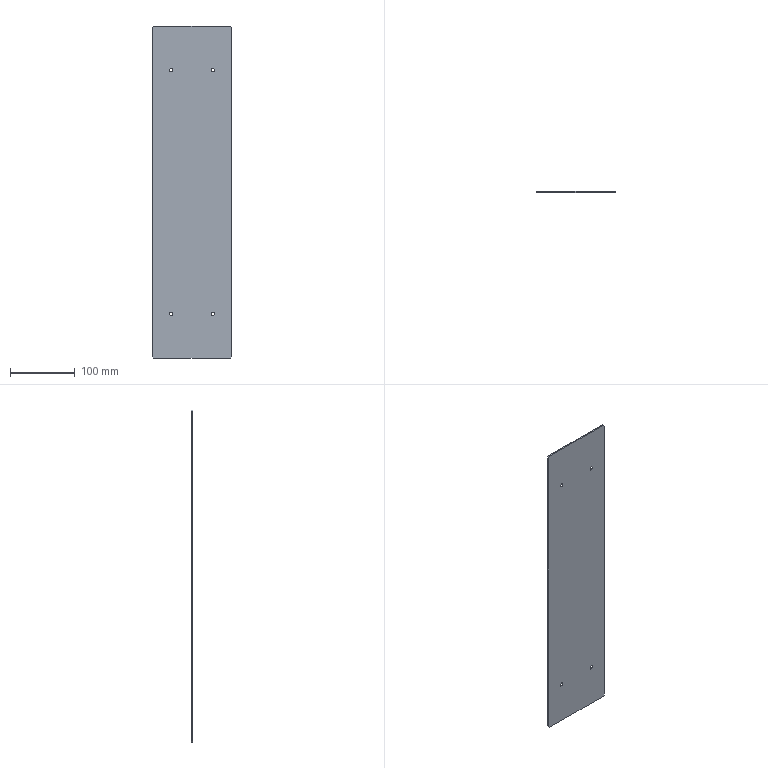Part | STEP file | (PA01.001.LX019) Cover Plate | 1 solid | 18 faces | box 123 x 2 x 511 mm | volume 125357 mm3 | plane 10 | cone 8
STEP:
#1=CARTESIAN_POINT('',(0.,0.,0.));
#2=DIRECTION('',(0.,0.,1.));
#3=DIRECTION('',(1.,0.,0.));
#4=AXIS2_PLACEMENT_3D('',#1,#2,#3);
#5=CARTESIAN_POINT('',(29.5,-2.,70.48));
#6=VERTEX_POINT('',#5);
#7=CARTESIAN_POINT('',(29.5,0.,72.48));
#8=VERTEX_POINT('',#7);
#9=CARTESIAN_POINT('',(29.5,0.,72.48));
#10=DIRECTION('',(0.,0.7071,0.7071));
#11=VECTOR('',#10,1.);
#12=LINE('',#9,#11);
#13=CARTESIAN_POINT('',(29.5,0.,68.));
#14=DIRECTION('',(0.,1.,0.));
#15=DIRECTION('',(0.,0.,1.));
#16=AXIS2_PLACEMENT_3D('',#13,#14,#15);
#17=CONICAL_SURFACE('',#16,4.48,0.7854);
#18=CARTESIAN_POINT('',(6.283,0.));
#19=DIRECTION('',(0.,1.));
#20=VECTOR('',#19,1.);
#21=LINE('',#18,#20);
#22=(GEOMETRIC_REPRESENTATION_CONTEXT(2)PARAMETRIC_REPRESENTATION_CONTEXT()REPRESENTATION_CONTEXT('',''));
#23=DEFINITIONAL_REPRESENTATION('',(#21),#22);
#24=PCURVE('',#17,#23);
#25=CARTESIAN_POINT('',(29.5,0.,68.));
#26=DIRECTION('',(0.,1.,0.));
#27=DIRECTION('',(0.,0.,1.));
#28=AXIS2_PLACEMENT_3D('',#25,#26,#27);
#29=CONICAL_SURFACE('',#28,4.48,0.7854);
#30=CARTESIAN_POINT('',(0.,0.));
#31=DIRECTION('',(0.,1.));
#32=VECTOR('',#31,1.);
#33=LINE('',#30,#32);
#34=(GEOMETRIC_REPRESENTATION_CONTEXT(2)PARAMETRIC_REPRESENTATION_CONTEXT()REPRESENTATION_CONTEXT('',''));
#35=DEFINITIONAL_REPRESENTATION('',(#33),#34);
#36=PCURVE('',#29,#35);
#37=SURFACE_CURVE('',#12,(#24,#36),.PCURVE_S1.);
#38=EDGE_CURVE('',#6,#8,#37,.T.);
#39=ORIENTED_EDGE('',*,*,#38,.T.);
#40=CARTESIAN_POINT('',(29.5,0.,63.52));
#41=VERTEX_POINT('',#40);
#42=CARTESIAN_POINT('',(29.5,0.,68.));
#43=DIRECTION('',(0.,1.,0.));
#44=DIRECTION('',(0.,0.,1.));
#45=AXIS2_PLACEMENT_3D('',#42,#43,#44);
#46=CIRCLE('',#45,4.48);
#47=CARTESIAN_POINT('',(0.,0.));
#48=DIRECTION('',(1.,0.));
#49=VECTOR('',#48,1.);
#50=LINE('',#47,#49);
#51=(GEOMETRIC_REPRESENTATION_CONTEXT(2)PARAMETRIC_REPRESENTATION_CONTEXT()REPRESENTATION_CONTEXT('',''));
#52=DEFINITIONAL_REPRESENTATION('',(#50),#51);
#53=PCURVE('',#17,#52);
#54=CARTESIAN_POINT('',(0.,0.,511.));
#55=DIRECTION('',(0.,1.,0.));
#56=DIRECTION('',(0.,0.,1.));
#57=AXIS2_PLACEMENT_3D('',#54,#55,#56);
#58=PLANE('',#57);
#59=CARTESIAN_POINT('',(-443.,29.5));
#60=DIRECTION('',(1.,0.));
#61=AXIS2_PLACEMENT_2D('',#59,#60);
#62=CIRCLE('',#61,4.48);
#63=(GEOMETRIC_REPRESENTATION_CONTEXT(2)PARAMETRIC_REPRESENTATION_CONTEXT()REPRESENTATION_CONTEXT('',''));
#64=DEFINITIONAL_REPRESENTATION('',(#62),#63);
#65=PCURVE('',#58,#64);
#66=SURFACE_CURVE('',#46,(#53,#65),.PCURVE_S1.);
#67=EDGE_CURVE('',#41,#8,#66,.T.);
#68=ORIENTED_EDGE('',*,*,#67,.F.);
#69=CARTESIAN_POINT('',(29.5,-2.,65.52));
#70=VERTEX_POINT('',#69);
#71=CARTESIAN_POINT('',(29.5,0.,63.52));
#72=DIRECTION('',(0.,0.7071,-0.7071));
#73=VECTOR('',#72,1.);
#74=LINE('',#71,#73);
#75=CARTESIAN_POINT('',(3.142,0.));
#76=DIRECTION('',(0.,1.));
#77=VECTOR('',#76,1.);
#78=LINE('',#75,#77);
#79=(GEOMETRIC_REPRESENTATION_CONTEXT(2)PARAMETRIC_REPRESENTATION_CONTEXT()REPRESENTATION_CONTEXT('',''));
#80=DEFINITIONAL_REPRESENTATION('',(#78),#79);
#81=PCURVE('',#17,#80);
#82=CARTESIAN_POINT('',(3.142,0.));
#83=DIRECTION('',(0.,1.));
#84=VECTOR('',#83,1.);
#85=LINE('',#82,#84);
#86=(GEOMETRIC_REPRESENTATION_CONTEXT(2)PARAMETRIC_REPRESENTATION_CONTEXT()REPRESENTATION_CONTEXT('',''));
#87=DEFINITIONAL_REPRESENTATION('',(#85),#86);
#88=PCURVE('',#29,#87);
#89=SURFACE_CURVE('',#74,(#81,#88),.PCURVE_S1.);
#90=EDGE_CURVE('',#70,#41,#89,.T.);
#91=ORIENTED_EDGE('',*,*,#90,.F.);
#92=CARTESIAN_POINT('',(29.5,-2.,68.));
#93=DIRECTION('',(0.,1.,0.));
#94=DIRECTION('',(0.,0.,1.));
#95=AXIS2_PLACEMENT_3D('',#92,#93,#94);
#96=CIRCLE('',#95,2.48);
#97=CARTESIAN_POINT('',(0.,-2.));
#98=DIRECTION('',(1.,0.));
#99=VECTOR('',#98,1.);
#100=LINE('',#97,#99);
#101=(GEOMETRIC_REPRESENTATION_CONTEXT(2)PARAMETRIC_REPRESENTATION_CONTEXT()REPRESENTATION_CONTEXT('',''));
#102=DEFINITIONAL_REPRESENTATION('',(#100),#101);
#103=PCURVE('',#17,#102);
#104=CARTESIAN_POINT('',(0.,-2.,511.));
#105=DIRECTION('',(0.,1.,0.));
#106=DIRECTION('',(0.,0.,1.));
#107=AXIS2_PLACEMENT_3D('',#104,#105,#106);
#108=PLANE('',#107);
#109=CARTESIAN_POINT('',(-443.,29.5));
#110=DIRECTION('',(1.,0.));
#111=AXIS2_PLACEMENT_2D('',#109,#110);
#112=CIRCLE('',#111,2.48);
#113=(GEOMETRIC_REPRESENTATION_CONTEXT(2)PARAMETRIC_REPRESENTATION_CONTEXT()REPRESENTATION_CONTEXT('',''));
#114=DEFINITIONAL_REPRESENTATION('',(#112),#113);
#115=PCURVE('',#108,#114);
#116=SURFACE_CURVE('',#96,(#103,#115),.PCURVE_S1.);
#117=EDGE_CURVE('',#70,#6,#116,.T.);
#118=ORIENTED_EDGE('',*,*,#117,.T.);
#119=EDGE_LOOP('',(#39,#68,#91,#118));
#120=FACE_BOUND('',#119,.F.);
#121=ADVANCED_FACE('',(#120),#17,.F.);
#122=CARTESIAN_POINT('',(93.5,-2.,70.48));
#123=VERTEX_POINT('',#122);
#124=CARTESIAN_POINT('',(93.5,0.,72.48));
#125=VERTEX_POINT('',#124);
#126=CARTESIAN_POINT('',(93.5,0.,72.48));
#127=DIRECTION('',(0.,0.7071,0.7071));
#128=VECTOR('',#127,1.);
#129=LINE('',#126,#128);
#130=CARTESIAN_POINT('',(93.5,0.,68.));
#131=DIRECTION('',(0.,1.,0.));
#132=DIRECTION('',(0.,0.,1.));
#133=AXIS2_PLACEMENT_3D('',#130,#131,#132);
#134=CONICAL_SURFACE('',#133,4.48,0.7854);
#135=CARTESIAN_POINT('',(6.283,0.));
#136=DIRECTION('',(0.,1.));
#137=VECTOR('',#136,1.);
#138=LINE('',#135,#137);
#139=(GEOMETRIC_REPRESENTATION_CONTEXT(2)PARAMETRIC_REPRESENTATION_CONTEXT()REPRESENTATION_CONTEXT('',''));
#140=DEFINITIONAL_REPRESENTATION('',(#138),#139);
#141=PCURVE('',#134,#140);
#142=CARTESIAN_POINT('',(93.5,0.,68.));
#143=DIRECTION('',(0.,1.,0.));
#144=DIRECTION('',(0.,0.,1.));
#145=AXIS2_PLACEMENT_3D('',#142,#143,#144);
#146=CONICAL_SURFACE('',#145,4.48,0.7854);
#147=CARTESIAN_POINT('',(0.,0.));
#148=DIRECTION('',(0.,1.));
#149=VECTOR('',#148,1.);
#150=LINE('',#147,#149);
#151=(GEOMETRIC_REPRESENTATION_CONTEXT(2)PARAMETRIC_REPRESENTATION_CONTEXT()REPRESENTATION_CONTEXT('',''));
#152=DEFINITIONAL_REPRESENTATION('',(#150),#151);
#153=PCURVE('',#146,#152);
#154=SURFACE_CURVE('',#129,(#141,#153),.PCURVE_S1.);
#155=EDGE_CURVE('',#123,#125,#154,.T.);
#156=ORIENTED_EDGE('',*,*,#155,.T.);
#157=CARTESIAN_POINT('',(93.5,0.,63.52));
#158=VERTEX_POINT('',#157);
#159=CARTESIAN_POINT('',(93.5,0.,68.));
#160=DIRECTION('',(0.,1.,0.));
#161=DIRECTION('',(0.,0.,1.));
#162=AXIS2_PLACEMENT_3D('',#159,#160,#161);
#163=CIRCLE('',#162,4.48);
#164=CARTESIAN_POINT('',(0.,0.));
#165=DIRECTION('',(1.,0.));
#166=VECTOR('',#165,1.);
#167=LINE('',#164,#166);
#168=(GEOMETRIC_REPRESENTATION_CONTEXT(2)PARAMETRIC_REPRESENTATION_CONTEXT()REPRESENTATION_CONTEXT('',''));
#169=DEFINITIONAL_REPRESENTATION('',(#167),#168);
#170=PCURVE('',#134,#169);
#171=CARTESIAN_POINT('',(-443.,93.5));
#172=DIRECTION('',(1.,0.));
#173=AXIS2_PLACEMENT_2D('',#171,#172);
#174=CIRCLE('',#173,4.48);
#175=(GEOMETRIC_REPRESENTATION_CONTEXT(2)PARAMETRIC_REPRESENTATION_CONTEXT()REPRESENTATION_CONTEXT('',''));
#176=DEFINITIONAL_REPRESENTATION('',(#174),#175);
#177=PCURVE('',#58,#176);
#178=SURFACE_CURVE('',#163,(#170,#177),.PCURVE_S1.);
#179=EDGE_CURVE('',#158,#125,#178,.T.);
#180=ORIENTED_EDGE('',*,*,#179,.F.);
#181=CARTESIAN_POINT('',(93.5,-2.,65.52));
#182=VERTEX_POINT('',#181);
#183=CARTESIAN_POINT('',(93.5,0.,63.52));
#184=DIRECTION('',(0.,0.7071,-0.7071));
#185=VECTOR('',#184,1.);
#186=LINE('',#183,#185);
#187=CARTESIAN_POINT('',(3.142,0.));
#188=DIRECTION('',(0.,1.));
#189=VECTOR('',#188,1.);
#190=LINE('',#187,#189);
#191=(GEOMETRIC_REPRESENTATION_CONTEXT(2)PARAMETRIC_REPRESENTATION_CONTEXT()REPRESENTATION_CONTEXT('',''));
#192=DEFINITIONAL_REPRESENTATION('',(#190),#191);
#193=PCURVE('',#134,#192);
#194=CARTESIAN_POINT('',(3.142,0.));
#195=DIRECTION('',(0.,1.));
#196=VECTOR('',#195,1.);
#197=LINE('',#194,#196);
#198=(GEOMETRIC_REPRESENTATION_CONTEXT(2)PARAMETRIC_REPRESENTATION_CONTEXT()REPRESENTATION_CONTEXT('',''));
#199=DEFINITIONAL_REPRESENTATION('',(#197),#198);
#200=PCURVE('',#146,#199);
#201=SURFACE_CURVE('',#186,(#193,#200),.PCURVE_S1.);
#202=EDGE_CURVE('',#182,#158,#201,.T.);
#203=ORIENTED_EDGE('',*,*,#202,.F.);
#204=CARTESIAN_POINT('',(93.5,-2.,68.));
#205=DIRECTION('',(0.,1.,0.));
#206=DIRECTION('',(0.,0.,1.));
#207=AXIS2_PLACEMENT_3D('',#204,#205,#206);
#208=CIRCLE('',#207,2.48);
#209=CARTESIAN_POINT('',(0.,-2.));
#210=DIRECTION('',(1.,0.));
#211=VECTOR('',#210,1.);
#212=LINE('',#209,#211);
#213=(GEOMETRIC_REPRESENTATION_CONTEXT(2)PARAMETRIC_REPRESENTATION_CONTEXT()REPRESENTATION_CONTEXT('',''));
#214=DEFINITIONAL_REPRESENTATION('',(#212),#213);
#215=PCURVE('',#134,#214);
#216=CARTESIAN_POINT('',(-443.,93.5));
#217=DIRECTION('',(1.,0.));
#218=AXIS2_PLACEMENT_2D('',#216,#217);
#219=CIRCLE('',#218,2.48);
#220=(GEOMETRIC_REPRESENTATION_CONTEXT(2)PARAMETRIC_REPRESENTATION_CONTEXT()REPRESENTATION_CONTEXT('',''));
#221=DEFINITIONAL_REPRESENTATION('',(#219),#220);
#222=PCURVE('',#108,#221);
#223=SURFACE_CURVE('',#208,(#215,#222),.PCURVE_S1.);
#224=EDGE_CURVE('',#182,#123,#223,.T.);
#225=ORIENTED_EDGE('',*,*,#224,.T.);
#226=EDGE_LOOP('',(#156,#180,#203,#225));
#227=FACE_BOUND('',#226,.F.);
#228=ADVANCED_FACE('',(#227),#134,.F.);
#229=CARTESIAN_POINT('',(29.5,-2.,445.48));
#230=VERTEX_POINT('',#229);
#231=CARTESIAN_POINT('',(29.5,0.,447.48));
#232=VERTEX_POINT('',#231);
#233=CARTESIAN_POINT('',(29.5,0.,447.48));
#234=DIRECTION('',(0.,0.7071,0.7071));
#235=VECTOR('',#234,1.);
#236=LINE('',#233,#235);
#237=CARTESIAN_POINT('',(29.5,0.,443.));
#238=DIRECTION('',(0.,1.,0.));
#239=DIRECTION('',(0.,0.,1.));
#240=AXIS2_PLACEMENT_3D('',#237,#238,#239);
#241=CONICAL_SURFACE('',#240,4.48,0.7854);
#242=CARTESIAN_POINT('',(6.283,0.));
#243=DIRECTION('',(0.,1.));
#244=VECTOR('',#243,1.);
#245=LINE('',#242,#244);
#246=(GEOMETRIC_REPRESENTATION_CONTEXT(2)PARAMETRIC_REPRESENTATION_CONTEXT()REPRESENTATION_CONTEXT('',''));
#247=DEFINITIONAL_REPRESENTATION('',(#245),#246);
#248=PCURVE('',#241,#247);
#249=CARTESIAN_POINT('',(29.5,0.,443.));
#250=DIRECTION('',(0.,1.,0.));
#251=DIRECTION('',(0.,0.,1.));
#252=AXIS2_PLACEMENT_3D('',#249,#250,#251);
#253=CONICAL_SURFACE('',#252,4.48,0.7854);
#254=CARTESIAN_POINT('',(0.,0.));
#255=DIRECTION('',(0.,1.));
#256=VECTOR('',#255,1.);
#257=LINE('',#254,#256);
#258=(GEOMETRIC_REPRESENTATION_CONTEXT(2)PARAMETRIC_REPRESENTATION_CONTEXT()REPRESENTATION_CONTEXT('',''));
#259=DEFINITIONAL_REPRESENTATION('',(#257),#258);
#260=PCURVE('',#253,#259);
#261=SURFACE_CURVE('',#236,(#248,#260),.PCURVE_S1.);
#262=EDGE_CURVE('',#230,#232,#261,.T.);
#263=ORIENTED_EDGE('',*,*,#262,.T.);
#264=CARTESIAN_POINT('',(29.5,0.,438.52));
#265=VERTEX_POINT('',#264);
#266=CARTESIAN_POINT('',(29.5,0.,443.));
#267=DIRECTION('',(0.,1.,0.));
#268=DIRECTION('',(0.,0.,1.));
#269=AXIS2_PLACEMENT_3D('',#266,#267,#268);
#270=CIRCLE('',#269,4.48);
#271=CARTESIAN_POINT('',(0.,0.));
#272=DIRECTION('',(1.,0.));
#273=VECTOR('',#272,1.);
#274=LINE('',#271,#273);
#275=(GEOMETRIC_REPRESENTATION_CONTEXT(2)PARAMETRIC_REPRESENTATION_CONTEXT()REPRESENTATION_CONTEXT('',''));
#276=DEFINITIONAL_REPRESENTATION('',(#274),#275);
#277=PCURVE('',#241,#276);
#278=CARTESIAN_POINT('',(-68.,29.5));
#279=DIRECTION('',(1.,0.));
#280=AXIS2_PLACEMENT_2D('',#278,#279);
#281=CIRCLE('',#280,4.48);
#282=(GEOMETRIC_REPRESENTATION_CONTEXT(2)PARAMETRIC_REPRESENTATION_CONTEXT()REPRESENTATION_CONTEXT('',''));
#283=DEFINITIONAL_REPRESENTATION('',(#281),#282);
#284=PCURVE('',#58,#283);
#285=SURFACE_CURVE('',#270,(#277,#284),.PCURVE_S1.);
#286=EDGE_CURVE('',#265,#232,#285,.T.);
#287=ORIENTED_EDGE('',*,*,#286,.F.);
#288=CARTESIAN_POINT('',(29.5,-2.,440.52));
#289=VERTEX_POINT('',#288);
#290=CARTESIAN_POINT('',(29.5,0.,438.52));
#291=DIRECTION('',(0.,0.7071,-0.7071));
#292=VECTOR('',#291,1.);
#293=LINE('',#290,#292);
#294=CARTESIAN_POINT('',(3.142,0.));
#295=DIRECTION('',(0.,1.));
#296=VECTOR('',#295,1.);
#297=LINE('',#294,#296);
#298=(GEOMETRIC_REPRESENTATION_CONTEXT(2)PARAMETRIC_REPRESENTATION_CONTEXT()REPRESENTATION_CONTEXT('',''));
#299=DEFINITIONAL_REPRESENTATION('',(#297),#298);
#300=PCURVE('',#241,#299);
#301=CARTESIAN_POINT('',(3.142,0.));
#302=DIRECTION('',(0.,1.));
#303=VECTOR('',#302,1.);
#304=LINE('',#301,#303);
#305=(GEOMETRIC_REPRESENTATION_CONTEXT(2)PARAMETRIC_REPRESENTATION_CONTEXT()REPRESENTATION_CONTEXT('',''));
#306=DEFINITIONAL_REPRESENTATION('',(#304),#305);
#307=PCURVE('',#253,#306);
#308=SURFACE_CURVE('',#293,(#300,#307),.PCURVE_S1.);
#309=EDGE_CURVE('',#289,#265,#308,.T.);
#310=ORIENTED_EDGE('',*,*,#309,.F.);
#311=CARTESIAN_POINT('',(29.5,-2.,443.));
#312=DIRECTION('',(0.,1.,0.));
#313=DIRECTION('',(0.,0.,1.));
#314=AXIS2_PLACEMENT_3D('',#311,#312,#313);
#315=CIRCLE('',#314,2.48);
#316=CARTESIAN_POINT('',(0.,-2.));
#317=DIRECTION('',(1.,0.));
#318=VECTOR('',#317,1.);
#319=LINE('',#316,#318);
#320=(GEOMETRIC_REPRESENTATION_CONTEXT(2)PARAMETRIC_REPRESENTATION_CONTEXT()REPRESENTATION_CONTEXT('',''));
#321=DEFINITIONAL_REPRESENTATION('',(#319),#320);
#322=PCURVE('',#241,#321);
#323=CARTESIAN_POINT('',(-68.,29.5));
#324=DIRECTION('',(1.,0.));
#325=AXIS2_PLACEMENT_2D('',#323,#324);
#326=CIRCLE('',#325,2.48);
#327=(GEOMETRIC_REPRESENTATION_CONTEXT(2)PARAMETRIC_REPRESENTATION_CONTEXT()REPRESENTATION_CONTEXT('',''));
#328=DEFINITIONAL_REPRESENTATION('',(#326),#327);
#329=PCURVE('',#108,#328);
#330=SURFACE_CURVE('',#315,(#322,#329),.PCURVE_S1.);
#331=EDGE_CURVE('',#289,#230,#330,.T.);
#332=ORIENTED_EDGE('',*,*,#331,.T.);
#333=EDGE_LOOP('',(#263,#287,#310,#332));
#334=FACE_BOUND('',#333,.F.);
#335=ADVANCED_FACE('',(#334),#241,.F.);
#336=CARTESIAN_POINT('',(93.5,-2.,445.48));
#337=VERTEX_POINT('',#336);
#338=CARTESIAN_POINT('',(93.5,0.,447.48));
#339=VERTEX_POINT('',#338);
#340=CARTESIAN_POINT('',(93.5,0.,447.48));
#341=DIRECTION('',(0.,0.7071,0.7071));
#342=VECTOR('',#341,1.);
#343=LINE('',#340,#342);
#344=CARTESIAN_POINT('',(93.5,0.,443.));
#345=DIRECTION('',(0.,1.,0.));
#346=DIRECTION('',(0.,0.,1.));
#347=AXIS2_PLACEMENT_3D('',#344,#345,#346);
#348=CONICAL_SURFACE('',#347,4.48,0.7854);
#349=CARTESIAN_POINT('',(6.283,0.));
#350=DIRECTION('',(0.,1.));
#351=VECTOR('',#350,1.);
#352=LINE('',#349,#351);
#353=(GEOMETRIC_REPRESENTATION_CONTEXT(2)PARAMETRIC_REPRESENTATION_CONTEXT()REPRESENTATION_CONTEXT('',''));
#354=DEFINITIONAL_REPRESENTATION('',(#352),#353);
#355=PCURVE('',#348,#354);
#356=CARTESIAN_POINT('',(93.5,0.,443.));
#357=DIRECTION('',(0.,1.,0.));
#358=DIRECTION('',(0.,0.,1.));
#359=AXIS2_PLACEMENT_3D('',#356,#357,#358);
#360=CONICAL_SURFACE('',#359,4.48,0.7854);
#361=CARTESIAN_POINT('',(0.,0.));
#362=DIRECTION('',(0.,1.));
#363=VECTOR('',#362,1.);
#364=LINE('',#361,#363);
#365=(GEOMETRIC_REPRESENTATION_CONTEXT(2)PARAMETRIC_REPRESENTATION_CONTEXT()REPRESENTATION_CONTEXT('',''));
#366=DEFINITIONAL_REPRESENTATION('',(#364),#365);
#367=PCURVE('',#360,#366);
#368=SURFACE_CURVE('',#343,(#355,#367),.PCURVE_S1.);
#369=EDGE_CURVE('',#337,#339,#368,.T.);
#370=ORIENTED_EDGE('',*,*,#369,.T.);
#371=CARTESIAN_POINT('',(93.5,0.,438.52));
#372=VERTEX_POINT('',#371);
#373=CARTESIAN_POINT('',(93.5,0.,443.));
#374=DIRECTION('',(0.,1.,0.));
#375=DIRECTION('',(0.,0.,1.));
#376=AXIS2_PLACEMENT_3D('',#373,#374,#375);
#377=CIRCLE('',#376,4.48);
#378=CARTESIAN_POINT('',(0.,0.));
#379=DIRECTION('',(1.,0.));
#380=VECTOR('',#379,1.);
#381=LINE('',#378,#380);
#382=(GEOMETRIC_REPRESENTATION_CONTEXT(2)PARAMETRIC_REPRESENTATION_CONTEXT()REPRESENTATION_CONTEXT('',''));
#383=DEFINITIONAL_REPRESENTATION('',(#381),#382);
#384=PCURVE('',#348,#383);
#385=CARTESIAN_POINT('',(-68.,93.5));
#386=DIRECTION('',(1.,0.));
#387=AXIS2_PLACEMENT_2D('',#385,#386);
#388=CIRCLE('',#387,4.48);
#389=(GEOMETRIC_REPRESENTATION_CONTEXT(2)PARAMETRIC_REPRESENTATION_CONTEXT()REPRESENTATION_CONTEXT('',''));
#390=DEFINITIONAL_REPRESENTATION('',(#388),#389);
#391=PCURVE('',#58,#390);
#392=SURFACE_CURVE('',#377,(#384,#391),.PCURVE_S1.);
#393=EDGE_CURVE('',#372,#339,#392,.T.);
#394=ORIENTED_EDGE('',*,*,#393,.F.);
#395=CARTESIAN_POINT('',(93.5,-2.,440.52));
#396=VERTEX_POINT('',#395);
#397=CARTESIAN_POINT('',(93.5,0.,438.52));
#398=DIRECTION('',(0.,0.7071,-0.7071));
#399=VECTOR('',#398,1.);
#400=LINE('',#397,#399);
#401=CARTESIAN_POINT('',(3.142,0.));
#402=DIRECTION('',(0.,1.));
#403=VECTOR('',#402,1.);
#404=LINE('',#401,#403);
#405=(GEOMETRIC_REPRESENTATION_CONTEXT(2)PARAMETRIC_REPRESENTATION_CONTEXT()REPRESENTATION_CONTEXT('',''));
#406=DEFINITIONAL_REPRESENTATION('',(#404),#405);
#407=PCURVE('',#348,#406);
#408=CARTESIAN_POINT('',(3.142,0.));
#409=DIRECTION('',(0.,1.));
#410=VECTOR('',#409,1.);
#411=LINE('',#408,#410);
#412=(GEOMETRIC_REPRESENTATION_CONTEXT(2)PARAMETRIC_REPRESENTATION_CONTEXT()REPRESENTATION_CONTEXT('',''));
#413=DEFINITIONAL_REPRESENTATION('',(#411),#412);
#414=PCURVE('',#360,#413);
#415=SURFACE_CURVE('',#400,(#407,#414),.PCURVE_S1.);
#416=EDGE_CURVE('',#396,#372,#415,.T.);
#417=ORIENTED_EDGE('',*,*,#416,.F.);
#418=CARTESIAN_POINT('',(93.5,-2.,443.));
#419=DIRECTION('',(0.,1.,0.));
#420=DIRECTION('',(0.,0.,1.));
#421=AXIS2_PLACEMENT_3D('',#418,#419,#420);
#422=CIRCLE('',#421,2.48);
#423=CARTESIAN_POINT('',(0.,-2.));
#424=DIRECTION('',(1.,0.));
#425=VECTOR('',#424,1.);
#426=LINE('',#423,#425);
#427=(GEOMETRIC_REPRESENTATION_CONTEXT(2)PARAMETRIC_REPRESENTATION_CONTEXT()REPRESENTATION_CONTEXT('',''));
#428=DEFINITIONAL_REPRESENTATION('',(#426),#427);
#429=PCURVE('',#348,#428);
#430=CARTESIAN_POINT('',(-68.,93.5));
#431=DIRECTION('',(1.,0.));
#432=AXIS2_PLACEMENT_2D('',#430,#431);
#433=CIRCLE('',#432,2.48);
#434=(GEOMETRIC_REPRESENTATION_CONTEXT(2)PARAMETRIC_REPRESENTATION_CONTEXT()REPRESENTATION_CONTEXT('',''));
#435=DEFINITIONAL_REPRESENTATION('',(#433),#434);
#436=PCURVE('',#108,#435);
#437=SURFACE_CURVE('',#422,(#429,#436),.PCURVE_S1.);
#438=EDGE_CURVE('',#396,#337,#437,.T.);
#439=ORIENTED_EDGE('',*,*,#438,.T.);
#440=EDGE_LOOP('',(#370,#394,#417,#439));
#441=FACE_BOUND('',#440,.F.);
#442=ADVANCED_FACE('',(#441),#348,.F.);
#443=CARTESIAN_POINT('',(29.5,-2.,68.));
#444=DIRECTION('',(0.,1.,0.));
#445=DIRECTION('',(0.,0.,1.));
#446=AXIS2_PLACEMENT_3D('',#443,#444,#445);
#447=CIRCLE('',#446,2.48);
#448=CARTESIAN_POINT('',(-443.,29.5));
#449=DIRECTION('',(1.,0.));
#450=AXIS2_PLACEMENT_2D('',#448,#449);
#451=CIRCLE('',#450,2.48);
#452=(GEOMETRIC_REPRESENTATION_CONTEXT(2)PARAMETRIC_REPRESENTATION_CONTEXT()REPRESENTATION_CONTEXT('',''));
#453=DEFINITIONAL_REPRESENTATION('',(#451),#452);
#454=PCURVE('',#108,#453);
#455=CARTESIAN_POINT('',(0.,-2.));
#456=DIRECTION('',(1.,0.));
#457=VECTOR('',#456,1.);
#458=LINE('',#455,#457);
#459=(GEOMETRIC_REPRESENTATION_CONTEXT(2)PARAMETRIC_REPRESENTATION_CONTEXT()REPRESENTATION_CONTEXT('',''));
#460=DEFINITIONAL_REPRESENTATION('',(#458),#459);
#461=PCURVE('',#29,#460);
#462=SURFACE_CURVE('',#447,(#454,#461),.PCURVE_S1.);
#463=EDGE_CURVE('',#6,#70,#462,.T.);
#464=ORIENTED_EDGE('',*,*,#463,.T.);
#465=ORIENTED_EDGE('',*,*,#117,.T.);
#466=EDGE_LOOP('',(#464,#465));
#467=FACE_BOUND('',#466,.T.);
#468=CARTESIAN_POINT('',(93.5,-2.,68.));
#469=DIRECTION('',(0.,1.,0.));
#470=DIRECTION('',(0.,0.,1.));
#471=AXIS2_PLACEMENT_3D('',#468,#469,#470);
#472=CIRCLE('',#471,2.48);
#473=CARTESIAN_POINT('',(-443.,93.5));
#474=DIRECTION('',(1.,0.));
#475=AXIS2_PLACEMENT_2D('',#473,#474);
#476=CIRCLE('',#475,2.48);
#477=(GEOMETRIC_REPRESENTATION_CONTEXT(2)PARAMETRIC_REPRESENTATION_CONTEXT()REPRESENTATION_CONTEXT('',''));
#478=DEFINITIONAL_REPRESENTATION('',(#476),#477);
#479=PCURVE('',#108,#478);
#480=CARTESIAN_POINT('',(0.,-2.));
#481=DIRECTION('',(1.,0.));
#482=VECTOR('',#481,1.);
#483=LINE('',#480,#482);
#484=(GEOMETRIC_REPRESENTATION_CONTEXT(2)PARAMETRIC_REPRESENTATION_CONTEXT()REPRESENTATION_CONTEXT('',''));
#485=DEFINITIONAL_REPRESENTATION('',(#483),#484);
#486=PCURVE('',#146,#485);
#487=SURFACE_CURVE('',#472,(#479,#486),.PCURVE_S1.);
#488=EDGE_CURVE('',#123,#182,#487,.T.);
#489=ORIENTED_EDGE('',*,*,#488,.T.);
#490=ORIENTED_EDGE('',*,*,#224,.T.);
#491=EDGE_LOOP('',(#489,#490));
#492=FACE_BOUND('',#491,.T.);
#493=CARTESIAN_POINT('',(29.5,-2.,443.));
#494=DIRECTION('',(0.,1.,0.));
#495=DIRECTION('',(0.,0.,1.));
#496=AXIS2_PLACEMENT_3D('',#493,#494,#495);
#497=CIRCLE('',#496,2.48);
#498=CARTESIAN_POINT('',(-68.,29.5));
#499=DIRECTION('',(1.,0.));
#500=AXIS2_PLACEMENT_2D('',#498,#499);
#501=CIRCLE('',#500,2.48);
#502=(GEOMETRIC_REPRESENTATION_CONTEXT(2)PARAMETRIC_REPRESENTATION_CONTEXT()REPRESENTATION_CONTEXT('',''));
#503=DEFINITIONAL_REPRESENTATION('',(#501),#502);
#504=PCURVE('',#108,#503);
#505=CARTESIAN_POINT('',(0.,-2.));
#506=DIRECTION('',(1.,0.));
#507=VECTOR('',#506,1.);
#508=LINE('',#505,#507);
#509=(GEOMETRIC_REPRESENTATION_CONTEXT(2)PARAMETRIC_REPRESENTATION_CONTEXT()REPRESENTATION_CONTEXT('',''));
#510=DEFINITIONAL_REPRESENTATION('',(#508),#509);
#511=PCURVE('',#253,#510);
#512=SURFACE_CURVE('',#497,(#504,#511),.PCURVE_S1.);
#513=EDGE_CURVE('',#230,#289,#512,.T.);
#514=ORIENTED_EDGE('',*,*,#513,.T.);
#515=ORIENTED_EDGE('',*,*,#331,.T.);
#516=EDGE_LOOP('',(#514,#515));
#517=FACE_BOUND('',#516,.T.);
#518=CARTESIAN_POINT('',(0.,-2.,3.));
#519=VERTEX_POINT('',#518);
#520=CARTESIAN_POINT('',(0.,-2.,508.));
#521=VERTEX_POINT('',#520);
#522=CARTESIAN_POINT('',(0.,-2.,0.));
#523=DIRECTION('',(0.,0.,1.));
#524=VECTOR('',#523,1.);
#525=LINE('',#522,#524);
#526=CARTESIAN_POINT('',(-511.,0.));
#527=DIRECTION('',(1.,0.));
#528=VECTOR('',#527,1.);
#529=LINE('',#526,#528);
#530=(GEOMETRIC_REPRESENTATION_CONTEXT(2)PARAMETRIC_REPRESENTATION_CONTEXT()REPRESENTATION_CONTEXT('',''));
#531=DEFINITIONAL_REPRESENTATION('',(#529),#530);
#532=PCURVE('',#108,#531);
#533=CARTESIAN_POINT('',(0.,-2.,0.));
#534=DIRECTION('',(-1.,0.,0.));
#535=DIRECTION('',(0.,0.,1.));
#536=AXIS2_PLACEMENT_3D('',#533,#534,#535);
#537=PLANE('',#536);
#538=CARTESIAN_POINT('',(0.,0.));
#539=DIRECTION('',(1.,0.));
#540=VECTOR('',#539,1.);
#541=LINE('',#538,#540);
#542=(GEOMETRIC_REPRESENTATION_CONTEXT(2)PARAMETRIC_REPRESENTATION_CONTEXT()REPRESENTATION_CONTEXT('',''));
#543=DEFINITIONAL_REPRESENTATION('',(#541),#542);
#544=PCURVE('',#537,#543);
#545=SURFACE_CURVE('',#525,(#532,#544),.PCURVE_S1.);
#546=EDGE_CURVE('',#519,#521,#545,.T.);
#547=ORIENTED_EDGE('',*,*,#546,.F.);
#548=CARTESIAN_POINT('',(3.,-2.,0.));
#549=VERTEX_POINT('',#548);
#550=CARTESIAN_POINT('',(3.,-2.,0.));
#551=DIRECTION('',(0.7071,0.,-0.7071));
#552=VECTOR('',#551,1.);
#553=LINE('',#550,#552);
#554=CARTESIAN_POINT('',(-511.,3.));
#555=DIRECTION('',(-0.7071,0.7071));
#556=VECTOR('',#555,1.);
#557=LINE('',#554,#556);
#558=(GEOMETRIC_REPRESENTATION_CONTEXT(2)PARAMETRIC_REPRESENTATION_CONTEXT()REPRESENTATION_CONTEXT('',''));
#559=DEFINITIONAL_REPRESENTATION('',(#557),#558);
#560=PCURVE('',#108,#559);
#561=CARTESIAN_POINT('',(3.,-2.,0.));
#562=DIRECTION('',(0.7071,0.,0.7071));
#563=DIRECTION('',(0.7071,0.,-0.7071));
#564=AXIS2_PLACEMENT_3D('',#561,#562,#563);
#565=PLANE('',#564);
#566=CARTESIAN_POINT('',(0.,0.));
#567=DIRECTION('',(1.,0.));
#568=VECTOR('',#567,1.);
#569=LINE('',#566,#568);
#570=(GEOMETRIC_REPRESENTATION_CONTEXT(2)PARAMETRIC_REPRESENTATION_CONTEXT()REPRESENTATION_CONTEXT('',''));
#571=DEFINITIONAL_REPRESENTATION('',(#569),#570);
#572=PCURVE('',#565,#571);
#573=SURFACE_CURVE('',#553,(#560,#572),.PCURVE_S1.);
#574=EDGE_CURVE('',#519,#549,#573,.T.);
#575=ORIENTED_EDGE('',*,*,#574,.T.);
#576=CARTESIAN_POINT('',(120.,-2.,0.));
#577=VERTEX_POINT('',#576);
#578=CARTESIAN_POINT('',(0.,-2.,0.));
#579=DIRECTION('',(-1.,0.,0.));
#580=VECTOR('',#579,1.);
#581=LINE('',#578,#580);
#582=CARTESIAN_POINT('',(-511.,0.));
#583=DIRECTION('',(0.,-1.));
#584=VECTOR('',#583,1.);
#585=LINE('',#582,#584);
#586=(GEOMETRIC_REPRESENTATION_CONTEXT(2)PARAMETRIC_REPRESENTATION_CONTEXT()REPRESENTATION_CONTEXT('',''));
#587=DEFINITIONAL_REPRESENTATION('',(#585),#586);
#588=PCURVE('',#108,#587);
#589=CARTESIAN_POINT('',(0.,-2.,0.));
#590=DIRECTION('',(0.,0.,-1.));
#591=DIRECTION('',(-1.,0.,0.));
#592=AXIS2_PLACEMENT_3D('',#589,#590,#591);
#593=PLANE('',#592);
#594=CARTESIAN_POINT('',(0.,0.));
#595=DIRECTION('',(1.,0.));
#596=VECTOR('',#595,1.);
#597=LINE('',#594,#596);
#598=(GEOMETRIC_REPRESENTATION_CONTEXT(2)PARAMETRIC_REPRESENTATION_CONTEXT()REPRESENTATION_CONTEXT('',''));
#599=DEFINITIONAL_REPRESENTATION('',(#597),#598);
#600=PCURVE('',#593,#599);
#601=SURFACE_CURVE('',#581,(#588,#600),.PCURVE_S1.);
#602=EDGE_CURVE('',#577,#549,#601,.T.);
#603=ORIENTED_EDGE('',*,*,#602,.F.);
#604=CARTESIAN_POINT('',(123.,-2.,3.));
#605=VERTEX_POINT('',#604);
#606=CARTESIAN_POINT('',(123.,-2.,3.));
#607=DIRECTION('',(0.7071,0.,0.7071));
#608=VECTOR('',#607,1.);
#609=LINE('',#606,#608);
#610=CARTESIAN_POINT('',(-508.,123.));
#611=DIRECTION('',(0.7071,0.7071));
#612=VECTOR('',#611,1.);
#613=LINE('',#610,#612);
#614=(GEOMETRIC_REPRESENTATION_CONTEXT(2)PARAMETRIC_REPRESENTATION_CONTEXT()REPRESENTATION_CONTEXT('',''));
#615=DEFINITIONAL_REPRESENTATION('',(#613),#614);
#616=PCURVE('',#108,#615);
#617=CARTESIAN_POINT('',(123.,-2.,3.));
#618=DIRECTION('',(-0.7071,0.,0.7071));
#619=DIRECTION('',(0.7071,0.,0.7071));
#620=AXIS2_PLACEMENT_3D('',#617,#618,#619);
#621=PLANE('',#620);
#622=CARTESIAN_POINT('',(0.,0.));
#623=DIRECTION('',(1.,0.));
#624=VECTOR('',#623,1.);
#625=LINE('',#622,#624);
#626=(GEOMETRIC_REPRESENTATION_CONTEXT(2)PARAMETRIC_REPRESENTATION_CONTEXT()REPRESENTATION_CONTEXT('',''));
#627=DEFINITIONAL_REPRESENTATION('',(#625),#626);
#628=PCURVE('',#621,#627);
#629=SURFACE_CURVE('',#609,(#616,#628),.PCURVE_S1.);
#630=EDGE_CURVE('',#577,#605,#629,.T.);
#631=ORIENTED_EDGE('',*,*,#630,.T.);
#632=CARTESIAN_POINT('',(123.,-2.,508.));
#633=VERTEX_POINT('',#632);
#634=CARTESIAN_POINT('',(123.,-2.,0.));
#635=DIRECTION('',(0.,0.,-1.));
#636=VECTOR('',#635,1.);
#637=LINE('',#634,#636);
#638=CARTESIAN_POINT('',(-511.,123.));
#639=DIRECTION('',(-1.,0.));
#640=VECTOR('',#639,1.);
#641=LINE('',#638,#640);
#642=(GEOMETRIC_REPRESENTATION_CONTEXT(2)PARAMETRIC_REPRESENTATION_CONTEXT()REPRESENTATION_CONTEXT('',''));
#643=DEFINITIONAL_REPRESENTATION('',(#641),#642);
#644=PCURVE('',#108,#643);
#645=CARTESIAN_POINT('',(123.,-2.,0.));
#646=DIRECTION('',(1.,0.,0.));
#647=DIRECTION('',(0.,0.,-1.));
#648=AXIS2_PLACEMENT_3D('',#645,#646,#647);
#649=PLANE('',#648);
#650=CARTESIAN_POINT('',(0.,0.));
#651=DIRECTION('',(1.,0.));
#652=VECTOR('',#651,1.);
#653=LINE('',#650,#652);
#654=(GEOMETRIC_REPRESENTATION_CONTEXT(2)PARAMETRIC_REPRESENTATION_CONTEXT()REPRESENTATION_CONTEXT('',''));
#655=DEFINITIONAL_REPRESENTATION('',(#653),#654);
#656=PCURVE('',#649,#655);
#657=SURFACE_CURVE('',#637,(#644,#656),.PCURVE_S1.);
#658=EDGE_CURVE('',#633,#605,#657,.T.);
#659=ORIENTED_EDGE('',*,*,#658,.F.);
#660=CARTESIAN_POINT('',(120.,-2.,511.));
#661=VERTEX_POINT('',#660);
#662=CARTESIAN_POINT('',(120.,-2.,511.));
#663=DIRECTION('',(-0.7071,0.,0.7071));
#664=VECTOR('',#663,1.);
#665=LINE('',#662,#664);
#666=CARTESIAN_POINT('',(0.,120.));
#667=DIRECTION('',(0.7071,-0.7071));
#668=VECTOR('',#667,1.);
#669=LINE('',#666,#668);
#670=(GEOMETRIC_REPRESENTATION_CONTEXT(2)PARAMETRIC_REPRESENTATION_CONTEXT()REPRESENTATION_CONTEXT('',''));
#671=DEFINITIONAL_REPRESENTATION('',(#669),#670);
#672=PCURVE('',#108,#671);
#673=CARTESIAN_POINT('',(120.,-2.,511.));
#674=DIRECTION('',(-0.7071,0.,-0.7071));
#675=DIRECTION('',(-0.7071,0.,0.7071));
#676=AXIS2_PLACEMENT_3D('',#673,#674,#675);
#677=PLANE('',#676);
#678=CARTESIAN_POINT('',(0.,0.));
#679=DIRECTION('',(1.,0.));
#680=VECTOR('',#679,1.);
#681=LINE('',#678,#680);
#682=(GEOMETRIC_REPRESENTATION_CONTEXT(2)PARAMETRIC_REPRESENTATION_CONTEXT()REPRESENTATION_CONTEXT('',''));
#683=DEFINITIONAL_REPRESENTATION('',(#681),#682);
#684=PCURVE('',#677,#683);
#685=SURFACE_CURVE('',#665,(#672,#684),.PCURVE_S1.);
#686=EDGE_CURVE('',#633,#661,#685,.T.);
#687=ORIENTED_EDGE('',*,*,#686,.T.);
#688=CARTESIAN_POINT('',(3.,-2.,511.));
#689=VERTEX_POINT('',#688);
#690=CARTESIAN_POINT('',(0.,-2.,511.));
#691=DIRECTION('',(1.,0.,0.));
#692=VECTOR('',#691,1.);
#693=LINE('',#690,#692);
#694=CARTESIAN_POINT('',(0.,0.));
#695=DIRECTION('',(0.,1.));
#696=VECTOR('',#695,1.);
#697=LINE('',#694,#696);
#698=(GEOMETRIC_REPRESENTATION_CONTEXT(2)PARAMETRIC_REPRESENTATION_CONTEXT()REPRESENTATION_CONTEXT('',''));
#699=DEFINITIONAL_REPRESENTATION('',(#697),#698);
#700=PCURVE('',#108,#699);
#701=CARTESIAN_POINT('',(0.,-2.,511.));
#702=DIRECTION('',(0.,0.,1.));
#703=DIRECTION('',(1.,0.,0.));
#704=AXIS2_PLACEMENT_3D('',#701,#702,#703);
#705=PLANE('',#704);
#706=CARTESIAN_POINT('',(0.,0.));
#707=DIRECTION('',(1.,0.));
#708=VECTOR('',#707,1.);
#709=LINE('',#706,#708);
#710=(GEOMETRIC_REPRESENTATION_CONTEXT(2)PARAMETRIC_REPRESENTATION_CONTEXT()REPRESENTATION_CONTEXT('',''));
#711=DEFINITIONAL_REPRESENTATION('',(#709),#710);
#712=PCURVE('',#705,#711);
#713=SURFACE_CURVE('',#693,(#700,#712),.PCURVE_S1.);
#714=EDGE_CURVE('',#689,#661,#713,.T.);
#715=ORIENTED_EDGE('',*,*,#714,.F.);
#716=CARTESIAN_POINT('',(0.,-2.,508.));
#717=DIRECTION('',(-0.7071,0.,-0.7071));
#718=VECTOR('',#717,1.);
#719=LINE('',#716,#718);
#720=CARTESIAN_POINT('',(-3.,0.));
#721=DIRECTION('',(-0.7071,-0.7071));
#722=VECTOR('',#721,1.);
#723=LINE('',#720,#722);
#724=(GEOMETRIC_REPRESENTATION_CONTEXT(2)PARAMETRIC_REPRESENTATION_CONTEXT()REPRESENTATION_CONTEXT('',''));
#725=DEFINITIONAL_REPRESENTATION('',(#723),#724);
#726=PCURVE('',#108,#725);
#727=CARTESIAN_POINT('',(0.,-2.,508.));
#728=DIRECTION('',(0.7071,0.,-0.7071));
#729=DIRECTION('',(-0.7071,0.,-0.7071));
#730=AXIS2_PLACEMENT_3D('',#727,#728,#729);
#731=PLANE('',#730);
#732=CARTESIAN_POINT('',(0.,0.));
#733=DIRECTION('',(1.,0.));
#734=VECTOR('',#733,1.);
#735=LINE('',#732,#734);
#736=(GEOMETRIC_REPRESENTATION_CONTEXT(2)PARAMETRIC_REPRESENTATION_CONTEXT()REPRESENTATION_CONTEXT('',''));
#737=DEFINITIONAL_REPRESENTATION('',(#735),#736);
#738=PCURVE('',#731,#737);
#739=SURFACE_CURVE('',#719,(#726,#738),.PCURVE_S1.);
#740=EDGE_CURVE('',#689,#521,#739,.T.);
#741=ORIENTED_EDGE('',*,*,#740,.T.);
#742=EDGE_LOOP('',(#547,#575,#603,#631,#659,#687,#715,#741));
#743=FACE_BOUND('',#742,.T.);
#744=CARTESIAN_POINT('',(93.5,-2.,443.));
#745=DIRECTION('',(0.,1.,0.));
#746=DIRECTION('',(0.,0.,1.));
#747=AXIS2_PLACEMENT_3D('',#744,#745,#746);
#748=CIRCLE('',#747,2.48);
#749=CARTESIAN_POINT('',(-68.,93.5));
#750=DIRECTION('',(1.,0.));
#751=AXIS2_PLACEMENT_2D('',#749,#750);
#752=CIRCLE('',#751,2.48);
#753=(GEOMETRIC_REPRESENTATION_CONTEXT(2)PARAMETRIC_REPRESENTATION_CONTEXT()REPRESENTATION_CONTEXT('',''));
#754=DEFINITIONAL_REPRESENTATION('',(#752),#753);
#755=PCURVE('',#108,#754);
#756=CARTESIAN_POINT('',(0.,-2.));
#757=DIRECTION('',(1.,0.));
#758=VECTOR('',#757,1.);
#759=LINE('',#756,#758);
#760=(GEOMETRIC_REPRESENTATION_CONTEXT(2)PARAMETRIC_REPRESENTATION_CONTEXT()REPRESENTATION_CONTEXT('',''));
#761=DEFINITIONAL_REPRESENTATION('',(#759),#760);
#762=PCURVE('',#360,#761);
#763=SURFACE_CURVE('',#748,(#755,#762),.PCURVE_S1.);
#764=EDGE_CURVE('',#337,#396,#763,.T.);
#765=ORIENTED_EDGE('',*,*,#764,.T.);
#766=ORIENTED_EDGE('',*,*,#438,.T.);
#767=EDGE_LOOP('',(#765,#766));
#768=FACE_BOUND('',#767,.T.);
#769=ADVANCED_FACE('',(#467,#492,#517,#743,#768),#108,.F.);
#770=CARTESIAN_POINT('',(0.,0.,3.));
#771=VERTEX_POINT('',#770);
#772=CARTESIAN_POINT('',(0.,0.,508.));
#773=VERTEX_POINT('',#772);
#774=CARTESIAN_POINT('',(0.,0.,0.));
#775=DIRECTION('',(0.,0.,1.));
#776=VECTOR('',#775,1.);
#777=LINE('',#774,#776);
#778=CARTESIAN_POINT('',(0.,2.));
#779=DIRECTION('',(1.,0.));
#780=VECTOR('',#779,1.);
#781=LINE('',#778,#780);
#782=(GEOMETRIC_REPRESENTATION_CONTEXT(2)PARAMETRIC_REPRESENTATION_CONTEXT()REPRESENTATION_CONTEXT('',''));
#783=DEFINITIONAL_REPRESENTATION('',(#781),#782);
#784=PCURVE('',#537,#783);
#785=CARTESIAN_POINT('',(-511.,0.));
#786=DIRECTION('',(1.,0.));
#787=VECTOR('',#786,1.);
#788=LINE('',#785,#787);
#789=(GEOMETRIC_REPRESENTATION_CONTEXT(2)PARAMETRIC_REPRESENTATION_CONTEXT()REPRESENTATION_CONTEXT('',''));
#790=DEFINITIONAL_REPRESENTATION('',(#788),#789);
#791=PCURVE('',#58,#790);
#792=SURFACE_CURVE('',#777,(#784,#791),.PCURVE_S1.);
#793=EDGE_CURVE('',#771,#773,#792,.T.);
#794=ORIENTED_EDGE('',*,*,#793,.F.);
#795=CARTESIAN_POINT('',(0.,-2.,3.));
#796=DIRECTION('',(0.,-1.,0.));
#797=VECTOR('',#796,1.);
#798=LINE('',#795,#797);
#799=CARTESIAN_POINT('',(3.,0.));
#800=DIRECTION('',(0.,-1.));
#801=VECTOR('',#800,1.);
#802=LINE('',#799,#801);
#803=(GEOMETRIC_REPRESENTATION_CONTEXT(2)PARAMETRIC_REPRESENTATION_CONTEXT()REPRESENTATION_CONTEXT('',''));
#804=DEFINITIONAL_REPRESENTATION('',(#802),#803);
#805=PCURVE('',#537,#804);
#806=CARTESIAN_POINT('',(-4.243,0.));
#807=DIRECTION('',(0.,-1.));
#808=VECTOR('',#807,1.);
#809=LINE('',#806,#808);
#810=(GEOMETRIC_REPRESENTATION_CONTEXT(2)PARAMETRIC_REPRESENTATION_CONTEXT()REPRESENTATION_CONTEXT('',''));
#811=DEFINITIONAL_REPRESENTATION('',(#809),#810);
#812=PCURVE('',#565,#811);
#813=SURFACE_CURVE('',#798,(#805,#812),.PCURVE_S1.);
#814=EDGE_CURVE('',#771,#519,#813,.T.);
#815=ORIENTED_EDGE('',*,*,#814,.T.);
#816=ORIENTED_EDGE('',*,*,#546,.T.);
#817=CARTESIAN_POINT('',(0.,-2.,508.));
#818=DIRECTION('',(0.,1.,0.));
#819=VECTOR('',#818,1.);
#820=LINE('',#817,#819);
#821=CARTESIAN_POINT('',(508.,0.));
#822=DIRECTION('',(0.,1.));
#823=VECTOR('',#822,1.);
#824=LINE('',#821,#823);
#825=(GEOMETRIC_REPRESENTATION_CONTEXT(2)PARAMETRIC_REPRESENTATION_CONTEXT()REPRESENTATION_CONTEXT('',''));
#826=DEFINITIONAL_REPRESENTATION('',(#824),#825);
#827=PCURVE('',#537,#826);
#828=CARTESIAN_POINT('',(0.,0.));
#829=DIRECTION('',(0.,1.));
#830=VECTOR('',#829,1.);
#831=LINE('',#828,#830);
#832=(GEOMETRIC_REPRESENTATION_CONTEXT(2)PARAMETRIC_REPRESENTATION_CONTEXT()REPRESENTATION_CONTEXT('',''));
#833=DEFINITIONAL_REPRESENTATION('',(#831),#832);
#834=PCURVE('',#731,#833);
#835=SURFACE_CURVE('',#820,(#827,#834),.PCURVE_S1.);
#836=EDGE_CURVE('',#521,#773,#835,.T.);
#837=ORIENTED_EDGE('',*,*,#836,.T.);
#838=EDGE_LOOP('',(#794,#815,#816,#837));
#839=FACE_BOUND('',#838,.T.);
#840=ADVANCED_FACE('',(#839),#537,.T.);
#841=ORIENTED_EDGE('',*,*,#602,.T.);
#842=CARTESIAN_POINT('',(3.,0.,0.));
#843=VERTEX_POINT('',#842);
#844=CARTESIAN_POINT('',(3.,-2.,0.));
#845=DIRECTION('',(0.,1.,0.));
#846=VECTOR('',#845,1.);
#847=LINE('',#844,#846);
#848=CARTESIAN_POINT('',(-3.,0.));
#849=DIRECTION('',(0.,1.));
#850=VECTOR('',#849,1.);
#851=LINE('',#848,#850);
#852=(GEOMETRIC_REPRESENTATION_CONTEXT(2)PARAMETRIC_REPRESENTATION_CONTEXT()REPRESENTATION_CONTEXT('',''));
#853=DEFINITIONAL_REPRESENTATION('',(#851),#852);
#854=PCURVE('',#593,#853);
#855=CARTESIAN_POINT('',(0.,0.));
#856=DIRECTION('',(0.,1.));
#857=VECTOR('',#856,1.);
#858=LINE('',#855,#857);
#859=(GEOMETRIC_REPRESENTATION_CONTEXT(2)PARAMETRIC_REPRESENTATION_CONTEXT()REPRESENTATION_CONTEXT('',''));
#860=DEFINITIONAL_REPRESENTATION('',(#858),#859);
#861=PCURVE('',#565,#860);
#862=SURFACE_CURVE('',#847,(#854,#861),.PCURVE_S1.);
#863=EDGE_CURVE('',#549,#843,#862,.T.);
#864=ORIENTED_EDGE('',*,*,#863,.T.);
#865=CARTESIAN_POINT('',(120.,0.,0.));
#866=VERTEX_POINT('',#865);
#867=CARTESIAN_POINT('',(0.,0.,0.));
#868=DIRECTION('',(-1.,0.,0.));
#869=VECTOR('',#868,1.);
#870=LINE('',#867,#869);
#871=CARTESIAN_POINT('',(0.,2.));
#872=DIRECTION('',(1.,0.));
#873=VECTOR('',#872,1.);
#874=LINE('',#871,#873);
#875=(GEOMETRIC_REPRESENTATION_CONTEXT(2)PARAMETRIC_REPRESENTATION_CONTEXT()REPRESENTATION_CONTEXT('',''));
#876=DEFINITIONAL_REPRESENTATION('',(#874),#875);
#877=PCURVE('',#593,#876);
#878=CARTESIAN_POINT('',(-511.,0.));
#879=DIRECTION('',(0.,-1.));
#880=VECTOR('',#879,1.);
#881=LINE('',#878,#880);
#882=(GEOMETRIC_REPRESENTATION_CONTEXT(2)PARAMETRIC_REPRESENTATION_CONTEXT()REPRESENTATION_CONTEXT('',''));
#883=DEFINITIONAL_REPRESENTATION('',(#881),#882);
#884=PCURVE('',#58,#883);
#885=SURFACE_CURVE('',#870,(#877,#884),.PCURVE_S1.);
#886=EDGE_CURVE('',#866,#843,#885,.T.);
#887=ORIENTED_EDGE('',*,*,#886,.F.);
#888=CARTESIAN_POINT('',(120.,-2.,0.));
#889=DIRECTION('',(0.,-1.,0.));
#890=VECTOR('',#889,1.);
#891=LINE('',#888,#890);
#892=CARTESIAN_POINT('',(-120.,0.));
#893=DIRECTION('',(0.,-1.));
#894=VECTOR('',#893,1.);
#895=LINE('',#892,#894);
#896=(GEOMETRIC_REPRESENTATION_CONTEXT(2)PARAMETRIC_REPRESENTATION_CONTEXT()REPRESENTATION_CONTEXT('',''));
#897=DEFINITIONAL_REPRESENTATION('',(#895),#896);
#898=PCURVE('',#593,#897);
#899=CARTESIAN_POINT('',(-4.243,0.));
#900=DIRECTION('',(0.,-1.));
#901=VECTOR('',#900,1.);
#902=LINE('',#899,#901);
#903=(GEOMETRIC_REPRESENTATION_CONTEXT(2)PARAMETRIC_REPRESENTATION_CONTEXT()REPRESENTATION_CONTEXT('',''));
#904=DEFINITIONAL_REPRESENTATION('',(#902),#903);
#905=PCURVE('',#621,#904);
#906=SURFACE_CURVE('',#891,(#898,#905),.PCURVE_S1.);
#907=EDGE_CURVE('',#866,#577,#906,.T.);
#908=ORIENTED_EDGE('',*,*,#907,.T.);
#909=EDGE_LOOP('',(#841,#864,#887,#908));
#910=FACE_BOUND('',#909,.T.);
#911=ADVANCED_FACE('',(#910),#593,.T.);
#912=ORIENTED_EDGE('',*,*,#658,.T.);
#913=CARTESIAN_POINT('',(123.,0.,3.));
#914=VERTEX_POINT('',#913);
#915=CARTESIAN_POINT('',(123.,-2.,3.));
#916=DIRECTION('',(0.,1.,0.));
#917=VECTOR('',#916,1.);
#918=LINE('',#915,#917);
#919=CARTESIAN_POINT('',(-3.,0.));
#920=DIRECTION('',(0.,1.));
#921=VECTOR('',#920,1.);
#922=LINE('',#919,#921);
#923=(GEOMETRIC_REPRESENTATION_CONTEXT(2)PARAMETRIC_REPRESENTATION_CONTEXT()REPRESENTATION_CONTEXT('',''));
#924=DEFINITIONAL_REPRESENTATION('',(#922),#923);
#925=PCURVE('',#649,#924);
#926=CARTESIAN_POINT('',(0.,0.));
#927=DIRECTION('',(0.,1.));
#928=VECTOR('',#927,1.);
#929=LINE('',#926,#928);
#930=(GEOMETRIC_REPRESENTATION_CONTEXT(2)PARAMETRIC_REPRESENTATION_CONTEXT()REPRESENTATION_CONTEXT('',''));
#931=DEFINITIONAL_REPRESENTATION('',(#929),#930);
#932=PCURVE('',#621,#931);
#933=SURFACE_CURVE('',#918,(#925,#932),.PCURVE_S1.);
#934=EDGE_CURVE('',#605,#914,#933,.T.);
#935=ORIENTED_EDGE('',*,*,#934,.T.);
#936=CARTESIAN_POINT('',(123.,0.,508.));
#937=VERTEX_POINT('',#936);
#938=CARTESIAN_POINT('',(123.,0.,0.));
#939=DIRECTION('',(0.,0.,-1.));
#940=VECTOR('',#939,1.);
#941=LINE('',#938,#940);
#942=CARTESIAN_POINT('',(0.,2.));
#943=DIRECTION('',(1.,0.));
#944=VECTOR('',#943,1.);
#945=LINE('',#942,#944);
#946=(GEOMETRIC_REPRESENTATION_CONTEXT(2)PARAMETRIC_REPRESENTATION_CONTEXT()REPRESENTATION_CONTEXT('',''));
#947=DEFINITIONAL_REPRESENTATION('',(#945),#946);
#948=PCURVE('',#649,#947);
#949=CARTESIAN_POINT('',(-511.,123.));
#950=DIRECTION('',(-1.,0.));
#951=VECTOR('',#950,1.);
#952=LINE('',#949,#951);
#953=(GEOMETRIC_REPRESENTATION_CONTEXT(2)PARAMETRIC_REPRESENTATION_CONTEXT()REPRESENTATION_CONTEXT('',''));
#954=DEFINITIONAL_REPRESENTATION('',(#952),#953);
#955=PCURVE('',#58,#954);
#956=SURFACE_CURVE('',#941,(#948,#955),.PCURVE_S1.);
#957=EDGE_CURVE('',#937,#914,#956,.T.);
#958=ORIENTED_EDGE('',*,*,#957,.F.);
#959=CARTESIAN_POINT('',(123.,-2.,508.));
#960=DIRECTION('',(0.,-1.,0.));
#961=VECTOR('',#960,1.);
#962=LINE('',#959,#961);
#963=CARTESIAN_POINT('',(-508.,0.));
#964=DIRECTION('',(0.,-1.));
#965=VECTOR('',#964,1.);
#966=LINE('',#963,#965);
#967=(GEOMETRIC_REPRESENTATION_CONTEXT(2)PARAMETRIC_REPRESENTATION_CONTEXT()REPRESENTATION_CONTEXT('',''));
#968=DEFINITIONAL_REPRESENTATION('',(#966),#967);
#969=PCURVE('',#649,#968);
#970=CARTESIAN_POINT('',(-4.243,0.));
#971=DIRECTION('',(0.,-1.));
#972=VECTOR('',#971,1.);
#973=LINE('',#970,#972);
#974=(GEOMETRIC_REPRESENTATION_CONTEXT(2)PARAMETRIC_REPRESENTATION_CONTEXT()REPRESENTATION_CONTEXT('',''));
#975=DEFINITIONAL_REPRESENTATION('',(#973),#974);
#976=PCURVE('',#677,#975);
#977=SURFACE_CURVE('',#962,(#969,#976),.PCURVE_S1.);
#978=EDGE_CURVE('',#937,#633,#977,.T.);
#979=ORIENTED_EDGE('',*,*,#978,.T.);
#980=EDGE_LOOP('',(#912,#935,#958,#979));
#981=FACE_BOUND('',#980,.T.);
#982=ADVANCED_FACE('',(#981),#649,.T.);
#983=CARTESIAN_POINT('',(3.,0.,511.));
#984=VERTEX_POINT('',#983);
#985=CARTESIAN_POINT('',(120.,0.,511.));
#986=VERTEX_POINT('',#985);
#987=CARTESIAN_POINT('',(0.,0.,511.));
#988=DIRECTION('',(1.,0.,0.));
#989=VECTOR('',#988,1.);
#990=LINE('',#987,#989);
#991=CARTESIAN_POINT('',(0.,2.));
#992=DIRECTION('',(1.,0.));
#993=VECTOR('',#992,1.);
#994=LINE('',#991,#993);
#995=(GEOMETRIC_REPRESENTATION_CONTEXT(2)PARAMETRIC_REPRESENTATION_CONTEXT()REPRESENTATION_CONTEXT('',''));
#996=DEFINITIONAL_REPRESENTATION('',(#994),#995);
#997=PCURVE('',#705,#996);
#998=CARTESIAN_POINT('',(0.,0.));
#999=DIRECTION('',(0.,1.));
#1000=VECTOR('',#999,1.);
#1001=LINE('',#998,#1000);
#1002=(GEOMETRIC_REPRESENTATION_CONTEXT(2)PARAMETRIC_REPRESENTATION_CONTEXT()REPRESENTATION_CONTEXT('',''));
#1003=DEFINITIONAL_REPRESENTATION('',(#1001),#1002);
#1004=PCURVE('',#58,#1003);
#1005=SURFACE_CURVE('',#990,(#997,#1004),.PCURVE_S1.);
#1006=EDGE_CURVE('',#984,#986,#1005,.T.);
#1007=ORIENTED_EDGE('',*,*,#1006,.F.);
#1008=CARTESIAN_POINT('',(3.,-2.,511.));
#1009=DIRECTION('',(0.,-1.,0.));
#1010=VECTOR('',#1009,1.);
#1011=LINE('',#1008,#1010);
#1012=CARTESIAN_POINT('',(3.,0.));
#1013=DIRECTION('',(0.,-1.));
#1014=VECTOR('',#1013,1.);
#1015=LINE('',#1012,#1014);
#1016=(GEOMETRIC_REPRESENTATION_CONTEXT(2)PARAMETRIC_REPRESENTATION_CONTEXT()REPRESENTATION_CONTEXT('',''));
#1017=DEFINITIONAL_REPRESENTATION('',(#1015),#1016);
#1018=PCURVE('',#705,#1017);
#1019=CARTESIAN_POINT('',(-4.243,0.));
#1020=DIRECTION('',(0.,-1.));
#1021=VECTOR('',#1020,1.);
#1022=LINE('',#1019,#1021);
#1023=(GEOMETRIC_REPRESENTATION_CONTEXT(2)PARAMETRIC_REPRESENTATION_CONTEXT()REPRESENTATION_CONTEXT('',''));
#1024=DEFINITIONAL_REPRESENTATION('',(#1022),#1023);
#1025=PCURVE('',#731,#1024);
#1026=SURFACE_CURVE('',#1011,(#1018,#1025),.PCURVE_S1.);
#1027=EDGE_CURVE('',#984,#689,#1026,.T.);
#1028=ORIENTED_EDGE('',*,*,#1027,.T.);
#1029=ORIENTED_EDGE('',*,*,#714,.T.);
#1030=CARTESIAN_POINT('',(120.,-2.,511.));
#1031=DIRECTION('',(0.,1.,0.));
#1032=VECTOR('',#1031,1.);
#1033=LINE('',#1030,#1032);
#1034=CARTESIAN_POINT('',(120.,0.));
#1035=DIRECTION('',(0.,1.));
#1036=VECTOR('',#1035,1.);
#1037=LINE('',#1034,#1036);
#1038=(GEOMETRIC_REPRESENTATION_CONTEXT(2)PARAMETRIC_REPRESENTATION_CONTEXT()REPRESENTATION_CONTEXT('',''));
#1039=DEFINITIONAL_REPRESENTATION('',(#1037),#1038);
#1040=PCURVE('',#705,#1039);
#1041=CARTESIAN_POINT('',(0.,0.));
#1042=DIRECTION('',(0.,1.));
#1043=VECTOR('',#1042,1.);
#1044=LINE('',#1041,#1043);
#1045=(GEOMETRIC_REPRESENTATION_CONTEXT(2)PARAMETRIC_REPRESENTATION_CONTEXT()REPRESENTATION_CONTEXT('',''));
#1046=DEFINITIONAL_REPRESENTATION('',(#1044),#1045);
#1047=PCURVE('',#677,#1046);
#1048=SURFACE_CURVE('',#1033,(#1040,#1047),.PCURVE_S1.);
#1049=EDGE_CURVE('',#661,#986,#1048,.T.);
#1050=ORIENTED_EDGE('',*,*,#1049,.T.);
#1051=EDGE_LOOP('',(#1007,#1028,#1029,#1050));
#1052=FACE_BOUND('',#1051,.T.);
#1053=ADVANCED_FACE('',(#1052),#705,.T.);
#1054=CARTESIAN_POINT('',(29.5,0.,68.));
#1055=DIRECTION('',(0.,1.,0.));
#1056=DIRECTION('',(0.,0.,1.));
#1057=AXIS2_PLACEMENT_3D('',#1054,#1055,#1056);
#1058=CIRCLE('',#1057,4.48);
#1059=CARTESIAN_POINT('',(-443.,29.5));
#1060=DIRECTION('',(1.,0.));
#1061=AXIS2_PLACEMENT_2D('',#1059,#1060);
#1062=CIRCLE('',#1061,4.48);
#1063=(GEOMETRIC_REPRESENTATION_CONTEXT(2)PARAMETRIC_REPRESENTATION_CONTEXT()REPRESENTATION_CONTEXT('',''));
#1064=DEFINITIONAL_REPRESENTATION('',(#1062),#1063);
#1065=PCURVE('',#58,#1064);
#1066=CARTESIAN_POINT('',(0.,0.));
#1067=DIRECTION('',(1.,0.));
#1068=VECTOR('',#1067,1.);
#1069=LINE('',#1066,#1068);
#1070=(GEOMETRIC_REPRESENTATION_CONTEXT(2)PARAMETRIC_REPRESENTATION_CONTEXT()REPRESENTATION_CONTEXT('',''));
#1071=DEFINITIONAL_REPRESENTATION('',(#1069),#1070);
#1072=PCURVE('',#29,#1071);
#1073=SURFACE_CURVE('',#1058,(#1065,#1072),.PCURVE_S1.);
#1074=EDGE_CURVE('',#8,#41,#1073,.T.);
#1075=ORIENTED_EDGE('',*,*,#1074,.F.);
#1076=ORIENTED_EDGE('',*,*,#67,.F.);
#1077=EDGE_LOOP('',(#1075,#1076));
#1078=FACE_BOUND('',#1077,.T.);
#1079=CARTESIAN_POINT('',(93.5,0.,68.));
#1080=DIRECTION('',(0.,1.,0.));
#1081=DIRECTION('',(0.,0.,1.));
#1082=AXIS2_PLACEMENT_3D('',#1079,#1080,#1081);
#1083=CIRCLE('',#1082,4.48);
#1084=CARTESIAN_POINT('',(-443.,93.5));
#1085=DIRECTION('',(1.,0.));
#1086=AXIS2_PLACEMENT_2D('',#1084,#1085);
#1087=CIRCLE('',#1086,4.48);
#1088=(GEOMETRIC_REPRESENTATION_CONTEXT(2)PARAMETRIC_REPRESENTATION_CONTEXT()REPRESENTATION_CONTEXT('',''));
#1089=DEFINITIONAL_REPRESENTATION('',(#1087),#1088);
#1090=PCURVE('',#58,#1089);
#1091=CARTESIAN_POINT('',(0.,0.));
#1092=DIRECTION('',(1.,0.));
#1093=VECTOR('',#1092,1.);
#1094=LINE('',#1091,#1093);
#1095=(GEOMETRIC_REPRESENTATION_CONTEXT(2)PARAMETRIC_REPRESENTATION_CONTEXT()REPRESENTATION_CONTEXT('',''));
#1096=DEFINITIONAL_REPRESENTATION('',(#1094),#1095);
#1097=PCURVE('',#146,#1096);
#1098=SURFACE_CURVE('',#1083,(#1090,#1097),.PCURVE_S1.);
#1099=EDGE_CURVE('',#125,#158,#1098,.T.);
#1100=ORIENTED_EDGE('',*,*,#1099,.F.);
#1101=ORIENTED_EDGE('',*,*,#179,.F.);
#1102=EDGE_LOOP('',(#1100,#1101));
#1103=FACE_BOUND('',#1102,.T.);
#1104=CARTESIAN_POINT('',(29.5,0.,443.));
#1105=DIRECTION('',(0.,1.,0.));
#1106=DIRECTION('',(0.,0.,1.));
#1107=AXIS2_PLACEMENT_3D('',#1104,#1105,#1106);
#1108=CIRCLE('',#1107,4.48);
#1109=CARTESIAN_POINT('',(-68.,29.5));
#1110=DIRECTION('',(1.,0.));
#1111=AXIS2_PLACEMENT_2D('',#1109,#1110);
#1112=CIRCLE('',#1111,4.48);
#1113=(GEOMETRIC_REPRESENTATION_CONTEXT(2)PARAMETRIC_REPRESENTATION_CONTEXT()REPRESENTATION_CONTEXT('',''));
#1114=DEFINITIONAL_REPRESENTATION('',(#1112),#1113);
#1115=PCURVE('',#58,#1114);
#1116=CARTESIAN_POINT('',(0.,0.));
#1117=DIRECTION('',(1.,0.));
#1118=VECTOR('',#1117,1.);
#1119=LINE('',#1116,#1118);
#1120=(GEOMETRIC_REPRESENTATION_CONTEXT(2)PARAMETRIC_REPRESENTATION_CONTEXT()REPRESENTATION_CONTEXT('',''));
#1121=DEFINITIONAL_REPRESENTATION('',(#1119),#1120);
#1122=PCURVE('',#253,#1121);
#1123=SURFACE_CURVE('',#1108,(#1115,#1122),.PCURVE_S1.);
#1124=EDGE_CURVE('',#232,#265,#1123,.T.);
#1125=ORIENTED_EDGE('',*,*,#1124,.F.);
#1126=ORIENTED_EDGE('',*,*,#286,.F.);
#1127=EDGE_LOOP('',(#1125,#1126));
#1128=FACE_BOUND('',#1127,.T.);
#1129=CARTESIAN_POINT('',(93.5,0.,443.));
#1130=DIRECTION('',(0.,1.,0.));
#1131=DIRECTION('',(0.,0.,1.));
#1132=AXIS2_PLACEMENT_3D('',#1129,#1130,#1131);
#1133=CIRCLE('',#1132,4.48);
#1134=CARTESIAN_POINT('',(-68.,93.5));
#1135=DIRECTION('',(1.,0.));
#1136=AXIS2_PLACEMENT_2D('',#1134,#1135);
#1137=CIRCLE('',#1136,4.48);
#1138=(GEOMETRIC_REPRESENTATION_CONTEXT(2)PARAMETRIC_REPRESENTATION_CONTEXT()REPRESENTATION_CONTEXT('',''));
#1139=DEFINITIONAL_REPRESENTATION('',(#1137),#1138);
#1140=PCURVE('',#58,#1139);
#1141=CARTESIAN_POINT('',(0.,0.));
#1142=DIRECTION('',(1.,0.));
#1143=VECTOR('',#1142,1.);
#1144=LINE('',#1141,#1143);
#1145=(GEOMETRIC_REPRESENTATION_CONTEXT(2)PARAMETRIC_REPRESENTATION_CONTEXT()REPRESENTATION_CONTEXT('',''));
#1146=DEFINITIONAL_REPRESENTATION('',(#1144),#1145);
#1147=PCURVE('',#360,#1146);
#1148=SURFACE_CURVE('',#1133,(#1140,#1147),.PCURVE_S1.);
#1149=EDGE_CURVE('',#339,#372,#1148,.T.);
#1150=ORIENTED_EDGE('',*,*,#1149,.F.);
#1151=ORIENTED_EDGE('',*,*,#393,.F.);
#1152=EDGE_LOOP('',(#1150,#1151));
#1153=FACE_BOUND('',#1152,.T.);
#1154=ORIENTED_EDGE('',*,*,#886,.T.);
#1155=CARTESIAN_POINT('',(-254.,0.,257.));
#1156=DIRECTION('',(-0.7071,0.,0.7071));
#1157=VECTOR('',#1156,1.);
#1158=LINE('',#1155,#1157);
#1159=CARTESIAN_POINT('',(-254.,-254.));
#1160=DIRECTION('',(0.7071,-0.7071));
#1161=VECTOR('',#1160,1.);
#1162=LINE('',#1159,#1161);
#1163=(GEOMETRIC_REPRESENTATION_CONTEXT(2)PARAMETRIC_REPRESENTATION_CONTEXT()REPRESENTATION_CONTEXT('',''));
#1164=DEFINITIONAL_REPRESENTATION('',(#1162),#1163);
#1165=PCURVE('',#58,#1164);
#1166=CARTESIAN_POINT('',(-363.453,2.));
#1167=DIRECTION('',(-1.,0.));
#1168=VECTOR('',#1167,1.);
#1169=LINE('',#1166,#1168);
#1170=(GEOMETRIC_REPRESENTATION_CONTEXT(2)PARAMETRIC_REPRESENTATION_CONTEXT()REPRESENTATION_CONTEXT('',''));
#1171=DEFINITIONAL_REPRESENTATION('',(#1169),#1170);
#1172=PCURVE('',#565,#1171);
#1173=SURFACE_CURVE('',#1158,(#1165,#1172),.PCURVE_S1.);
#1174=EDGE_CURVE('',#843,#771,#1173,.T.);
#1175=ORIENTED_EDGE('',*,*,#1174,.T.);
#1176=ORIENTED_EDGE('',*,*,#793,.T.);
#1177=CARTESIAN_POINT('',(1.5,0.,509.5));
#1178=DIRECTION('',(0.7071,0.,0.7071));
#1179=VECTOR('',#1178,1.);
#1180=LINE('',#1177,#1179);
#1181=CARTESIAN_POINT('',(-1.5,1.5));
#1182=DIRECTION('',(0.7071,0.7071));
#1183=VECTOR('',#1182,1.);
#1184=LINE('',#1181,#1183);
#1185=(GEOMETRIC_REPRESENTATION_CONTEXT(2)PARAMETRIC_REPRESENTATION_CONTEXT()REPRESENTATION_CONTEXT('',''));
#1186=DEFINITIONAL_REPRESENTATION('',(#1184),#1185);
#1187=PCURVE('',#58,#1186);
#1188=CARTESIAN_POINT('',(-2.121,2.));
#1189=DIRECTION('',(-1.,0.));
#1190=VECTOR('',#1189,1.);
#1191=LINE('',#1188,#1190);
#1192=(GEOMETRIC_REPRESENTATION_CONTEXT(2)PARAMETRIC_REPRESENTATION_CONTEXT()REPRESENTATION_CONTEXT('',''));
#1193=DEFINITIONAL_REPRESENTATION('',(#1191),#1192);
#1194=PCURVE('',#731,#1193);
#1195=SURFACE_CURVE('',#1180,(#1187,#1194),.PCURVE_S1.);
#1196=EDGE_CURVE('',#773,#984,#1195,.T.);
#1197=ORIENTED_EDGE('',*,*,#1196,.T.);
#1198=ORIENTED_EDGE('',*,*,#1006,.T.);
#1199=CARTESIAN_POINT('',(60.,0.,571.));
#1200=DIRECTION('',(0.7071,0.,-0.7071));
#1201=VECTOR('',#1200,1.);
#1202=LINE('',#1199,#1201);
#1203=CARTESIAN_POINT('',(60.,60.));
#1204=DIRECTION('',(-0.7071,0.7071));
#1205=VECTOR('',#1204,1.);
#1206=LINE('',#1203,#1205);
#1207=(GEOMETRIC_REPRESENTATION_CONTEXT(2)PARAMETRIC_REPRESENTATION_CONTEXT()REPRESENTATION_CONTEXT('',''));
#1208=DEFINITIONAL_REPRESENTATION('',(#1206),#1207);
#1209=PCURVE('',#58,#1208);
#1210=CARTESIAN_POINT('',(84.853,2.));
#1211=DIRECTION('',(-1.,0.));
#1212=VECTOR('',#1211,1.);
#1213=LINE('',#1210,#1212);
#1214=(GEOMETRIC_REPRESENTATION_CONTEXT(2)PARAMETRIC_REPRESENTATION_CONTEXT()REPRESENTATION_CONTEXT('',''));
#1215=DEFINITIONAL_REPRESENTATION('',(#1213),#1214);
#1216=PCURVE('',#677,#1215);
#1217=SURFACE_CURVE('',#1202,(#1209,#1216),.PCURVE_S1.);
#1218=EDGE_CURVE('',#986,#937,#1217,.T.);
#1219=ORIENTED_EDGE('',*,*,#1218,.T.);
#1220=ORIENTED_EDGE('',*,*,#957,.T.);
#1221=CARTESIAN_POINT('',(315.5,0.,195.5));
#1222=DIRECTION('',(-0.7071,0.,-0.7071));
#1223=VECTOR('',#1222,1.);
#1224=LINE('',#1221,#1223);
#1225=CARTESIAN_POINT('',(-315.5,315.5));
#1226=DIRECTION('',(-0.7071,-0.7071));
#1227=VECTOR('',#1226,1.);
#1228=LINE('',#1225,#1227);
#1229=(GEOMETRIC_REPRESENTATION_CONTEXT(2)PARAMETRIC_REPRESENTATION_CONTEXT()REPRESENTATION_CONTEXT('',''));
#1230=DEFINITIONAL_REPRESENTATION('',(#1228),#1229);
#1231=PCURVE('',#58,#1230);
#1232=CARTESIAN_POINT('',(272.236,2.));
#1233=DIRECTION('',(-1.,0.));
#1234=VECTOR('',#1233,1.);
#1235=LINE('',#1232,#1234);
#1236=(GEOMETRIC_REPRESENTATION_CONTEXT(2)PARAMETRIC_REPRESENTATION_CONTEXT()REPRESENTATION_CONTEXT('',''));
#1237=DEFINITIONAL_REPRESENTATION('',(#1235),#1236);
#1238=PCURVE('',#621,#1237);
#1239=SURFACE_CURVE('',#1224,(#1231,#1238),.PCURVE_S1.);
#1240=EDGE_CURVE('',#914,#866,#1239,.T.);
#1241=ORIENTED_EDGE('',*,*,#1240,.T.);
#1242=EDGE_LOOP('',(#1154,#1175,#1176,#1197,#1198,#1219,#1220,#1241));
#1243=FACE_BOUND('',#1242,.T.);
#1244=ADVANCED_FACE('',(#1078,#1103,#1128,#1153,#1243),#58,.T.);
#1245=ORIENTED_EDGE('',*,*,#574,.F.);
#1246=ORIENTED_EDGE('',*,*,#814,.F.);
#1247=ORIENTED_EDGE('',*,*,#1174,.F.);
#1248=ORIENTED_EDGE('',*,*,#863,.F.);
#1249=EDGE_LOOP('',(#1245,#1246,#1247,#1248));
#1250=FACE_BOUND('',#1249,.T.);
#1251=ADVANCED_FACE('',(#1250),#565,.F.);
#1252=ORIENTED_EDGE('',*,*,#630,.F.);
#1253=ORIENTED_EDGE('',*,*,#907,.F.);
#1254=ORIENTED_EDGE('',*,*,#1240,.F.);
#1255=ORIENTED_EDGE('',*,*,#934,.F.);
#1256=EDGE_LOOP('',(#1252,#1253,#1254,#1255));
#1257=FACE_BOUND('',#1256,.T.);
#1258=ADVANCED_FACE('',(#1257),#621,.F.);
#1259=ORIENTED_EDGE('',*,*,#740,.F.);
#1260=ORIENTED_EDGE('',*,*,#1027,.F.);
#1261=ORIENTED_EDGE('',*,*,#1196,.F.);
#1262=ORIENTED_EDGE('',*,*,#836,.F.);
#1263=EDGE_LOOP('',(#1259,#1260,#1261,#1262));
#1264=FACE_BOUND('',#1263,.T.);
#1265=ADVANCED_FACE('',(#1264),#731,.F.);
#1266=ORIENTED_EDGE('',*,*,#686,.F.);
#1267=ORIENTED_EDGE('',*,*,#978,.F.);
#1268=ORIENTED_EDGE('',*,*,#1218,.F.);
#1269=ORIENTED_EDGE('',*,*,#1049,.F.);
#1270=EDGE_LOOP('',(#1266,#1267,#1268,#1269));
#1271=FACE_BOUND('',#1270,.T.);
#1272=ADVANCED_FACE('',(#1271),#677,.F.);
#1273=ORIENTED_EDGE('',*,*,#1149,.F.);
#1274=ORIENTED_EDGE('',*,*,#369,.F.);
#1275=ORIENTED_EDGE('',*,*,#764,.T.);
#1276=ORIENTED_EDGE('',*,*,#416,.T.);
#1277=EDGE_LOOP('',(#1273,#1274,#1275,#1276));
#1278=FACE_BOUND('',#1277,.F.);
#1279=ADVANCED_FACE('',(#1278),#360,.F.);
#1280=ORIENTED_EDGE('',*,*,#1124,.F.);
#1281=ORIENTED_EDGE('',*,*,#262,.F.);
#1282=ORIENTED_EDGE('',*,*,#513,.T.);
#1283=ORIENTED_EDGE('',*,*,#309,.T.);
#1284=EDGE_LOOP('',(#1280,#1281,#1282,#1283));
#1285=FACE_BOUND('',#1284,.F.);
#1286=ADVANCED_FACE('',(#1285),#253,.F.);
#1287=ORIENTED_EDGE('',*,*,#1099,.F.);
#1288=ORIENTED_EDGE('',*,*,#155,.F.);
#1289=ORIENTED_EDGE('',*,*,#488,.T.);
#1290=ORIENTED_EDGE('',*,*,#202,.T.);
#1291=EDGE_LOOP('',(#1287,#1288,#1289,#1290));
#1292=FACE_BOUND('',#1291,.F.);
#1293=ADVANCED_FACE('',(#1292),#146,.F.);
#1294=ORIENTED_EDGE('',*,*,#1074,.F.);
#1295=ORIENTED_EDGE('',*,*,#38,.F.);
#1296=ORIENTED_EDGE('',*,*,#463,.T.);
#1297=ORIENTED_EDGE('',*,*,#90,.T.);
#1298=EDGE_LOOP('',(#1294,#1295,#1296,#1297));
#1299=FACE_BOUND('',#1298,.F.);
#1300=ADVANCED_FACE('',(#1299),#29,.F.);
#1301=CLOSED_SHELL('',(#121,#228,#335,#442,#769,#840,#911,#982,#1053,#1244,#1251,#1258,#1265,#1272,#1279,#1286,#1293,#1300));
#1302=MANIFOLD_SOLID_BREP('',#1301);
#1303=(LENGTH_UNIT()NAMED_UNIT(*)SI_UNIT(.MILLI.,.METRE.));
#1304=UNCERTAINTY_MEASURE_WITH_UNIT(LENGTH_MEASURE(0.0000001),#1303,'','');
#1305=(NAMED_UNIT(*)PLANE_ANGLE_UNIT()SI_UNIT($,.RADIAN.));
#1306=(NAMED_UNIT(*)SI_UNIT($,.STERADIAN.)SOLID_ANGLE_UNIT());
#1307=(GEOMETRIC_REPRESENTATION_CONTEXT(3)GLOBAL_UNCERTAINTY_ASSIGNED_CONTEXT((#1304))GLOBAL_UNIT_ASSIGNED_CONTEXT((#1303,#1305,#1306))REPRESENTATION_CONTEXT('',''));
#1308=ADVANCED_BREP_SHAPE_REPRESENTATION('',(#4,#1302),#1307);